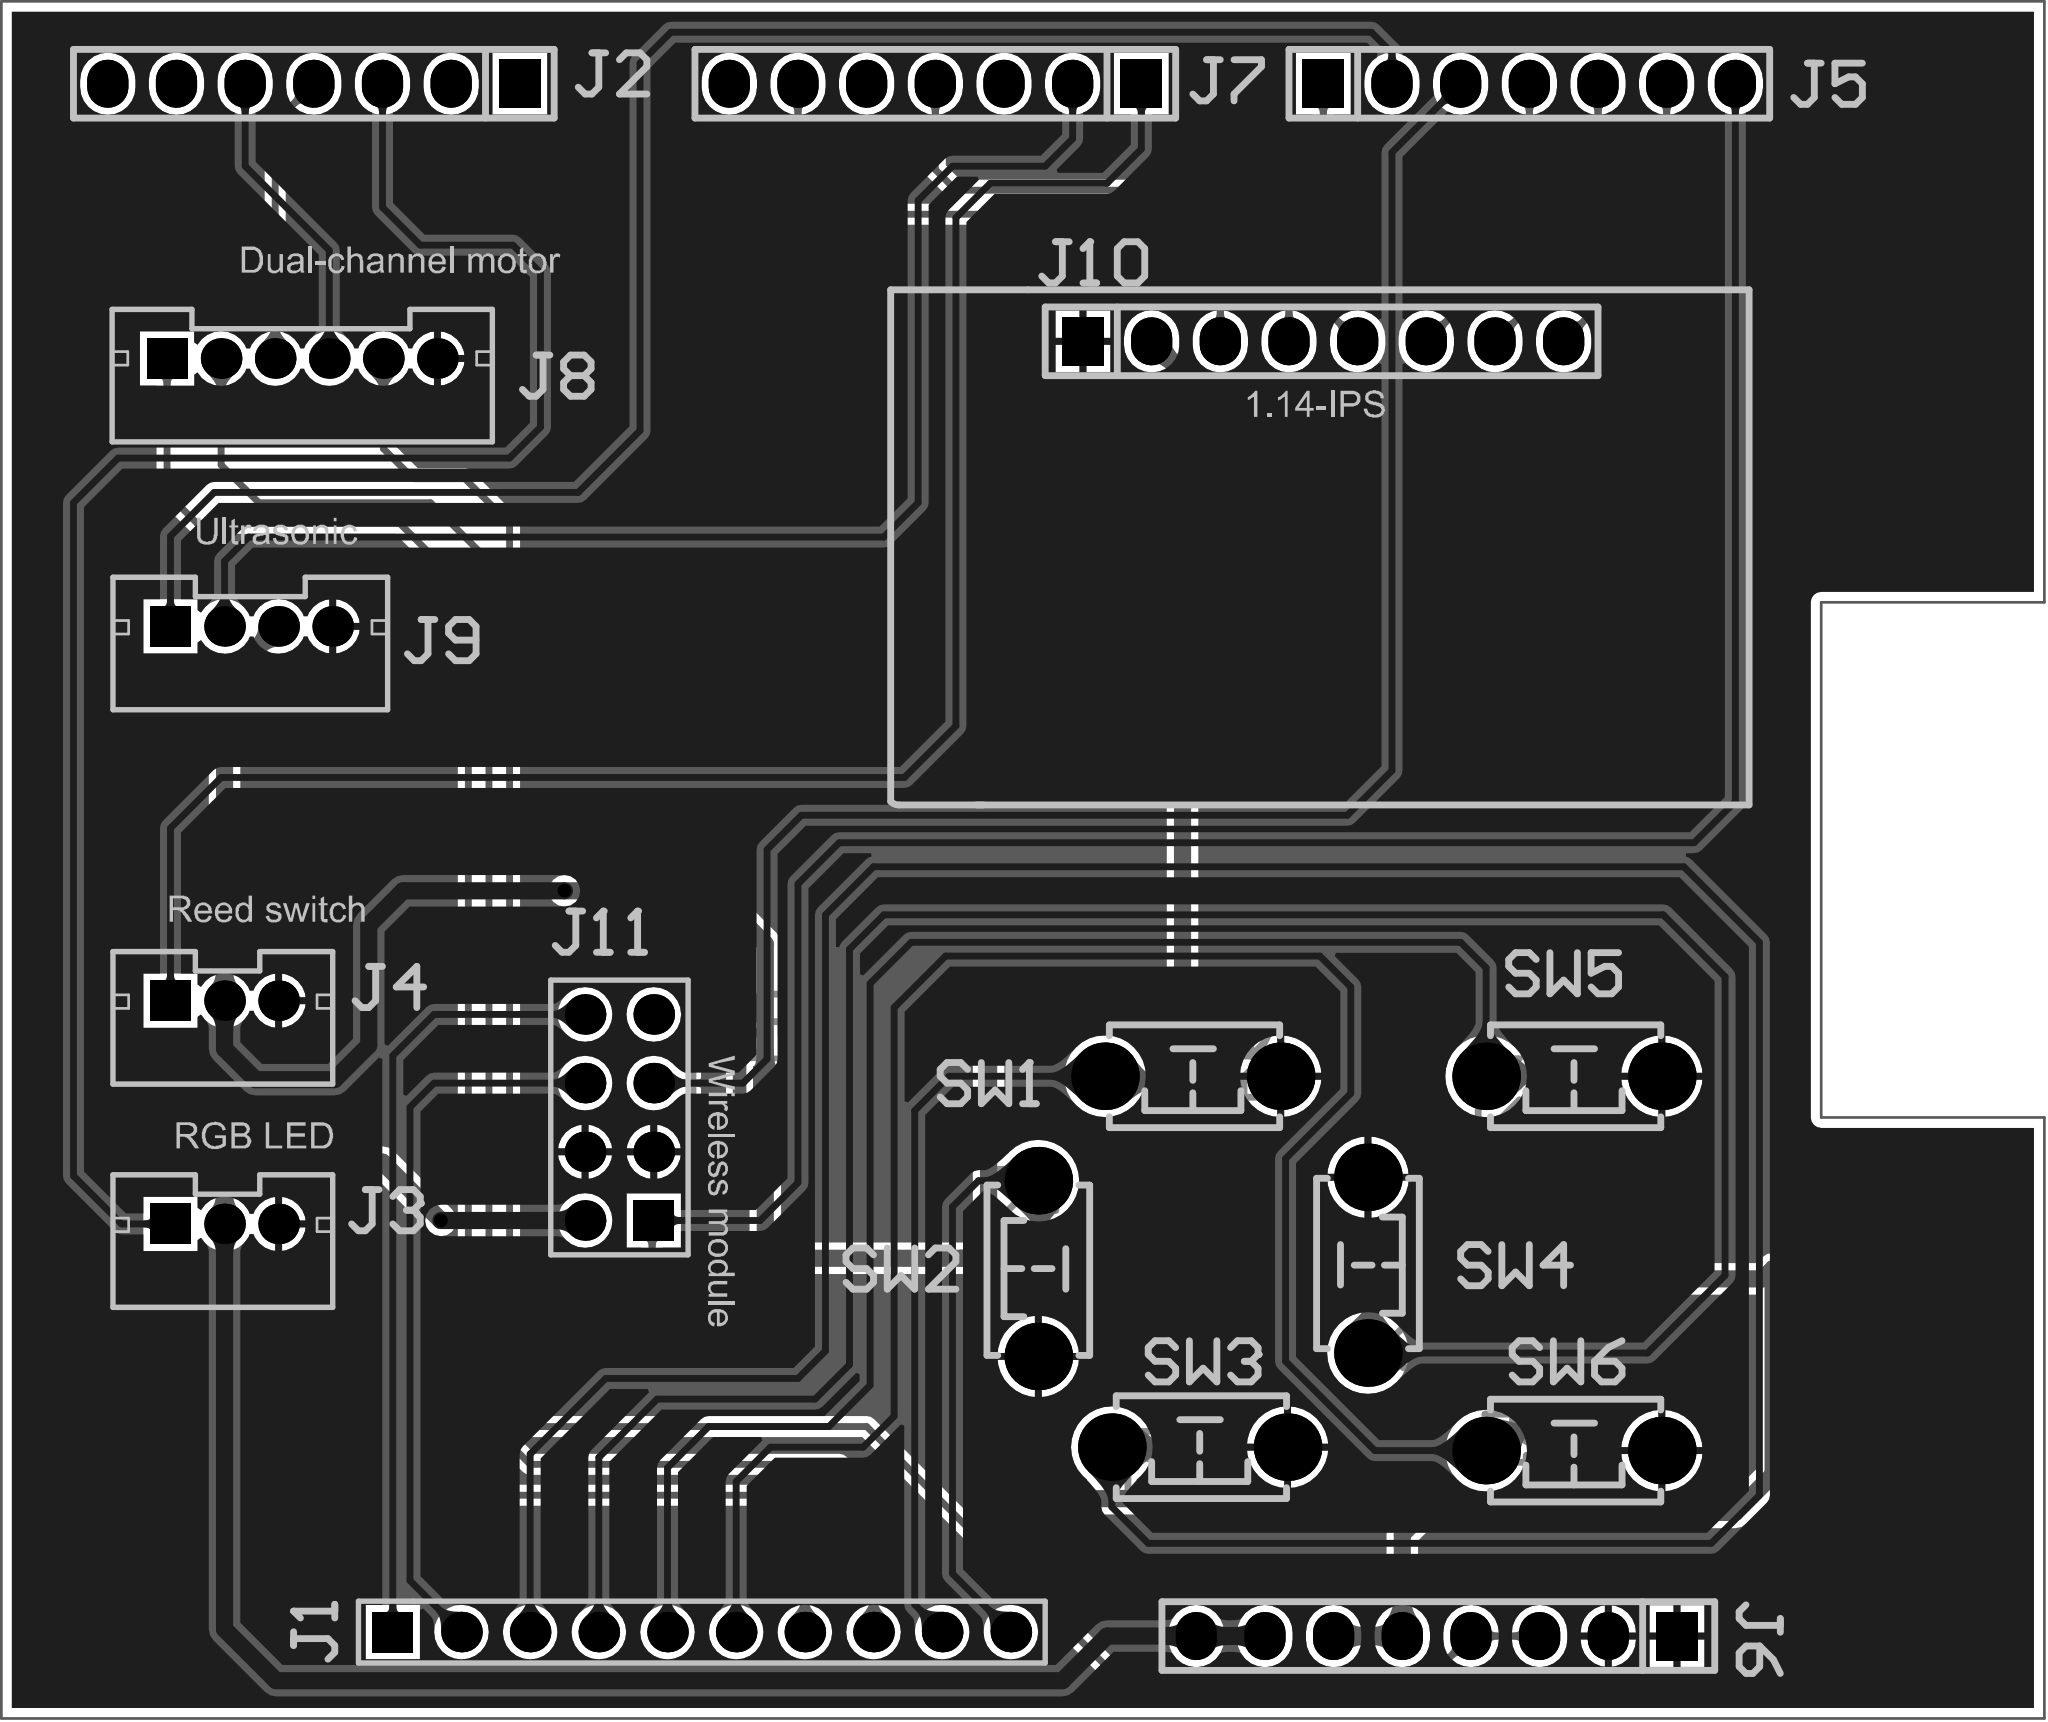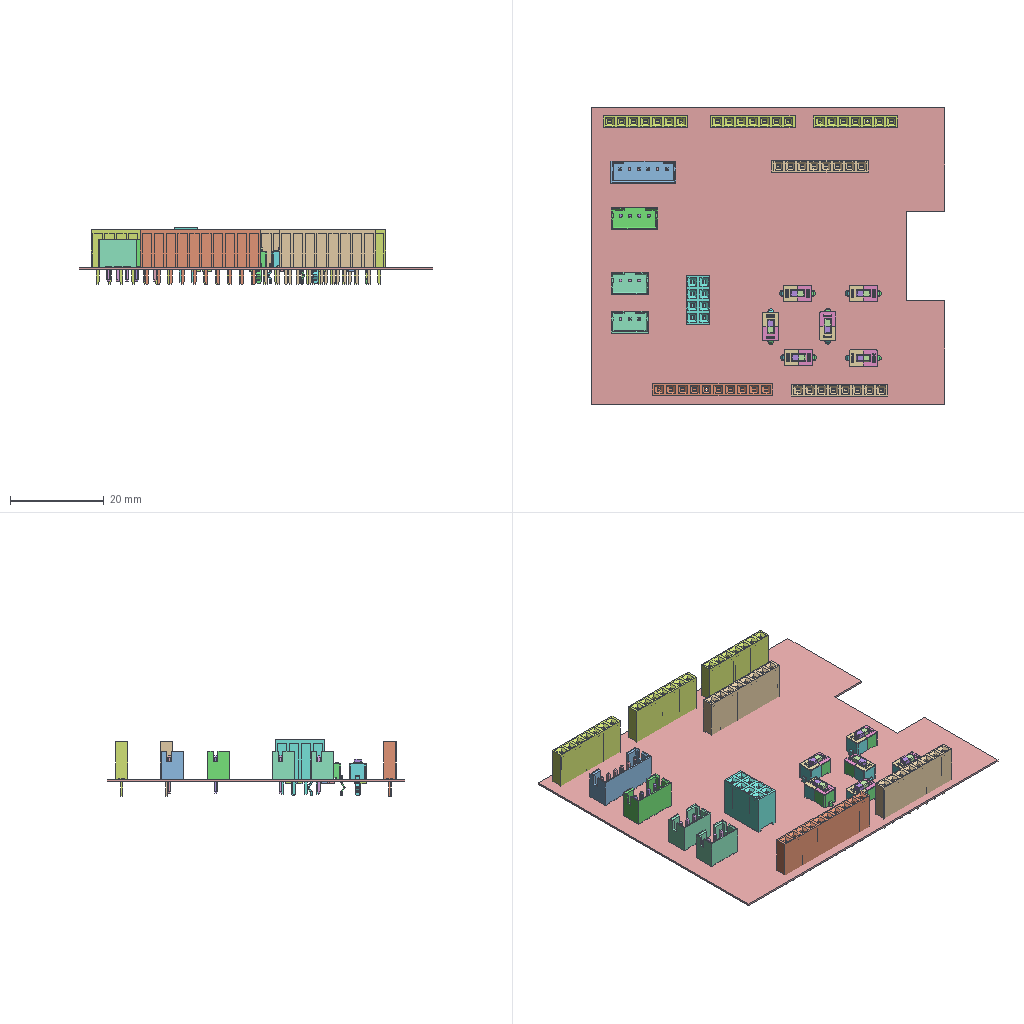Circuit board layout | Altium Designer | box 75.6 x 63.5 x 12.1 mm
Layer stack:
# Altium Designer layer stack of  (unit mm; dielectric type: 0 none, 1 core, 2 prepreg, 3 surface material)
index,name,kind,layer,copper_thickness_mm,dielectric_type,dielectric_thickness_mm,dielectric_material,dielectric_constant
0,Top Paste,other,,,,,,
1,Top Overlay,other,,,,,,
2,Top Solder,dielectric,,,3,0.0102,Solder Resist,3.5
3,Top Layer,copper,Top Layer,0.0356,,,,
4,Dielectric 1,dielectric,,,0,0.32,FR-4,4.8
5,Bottom Layer,copper,Bottom Layer,0.0356,,,,
6,Bottom Solder,dielectric,,,3,0.0102,Solder Resist,3.5
7,Bottom Overlay,other,,,,,,
8,Bottom Paste,other,,,,,,
# drill layer pairs: low layer,high layer
drill_pair,Top Layer,Bottom Layer
Part placement:
Designator,Comment,Layer,Footprint,Center-X(mm),Center-Y(mm),Rotation
SW6,3x6x5,TopLayer,TSW_DIP-3*6*4.3,97.536,46.101,180
SW5,3x6x5,TopLayer,TSW_DIP-3*6*4.3,97.536,59.944,180
SW4,3x6x5,TopLayer,TSW_DIP-3*6*4.3,89.916,52.959,270
SW3,3x6x5,TopLayer,TSW_DIP-3*6*4.3,83.693,46.228,180
SW2,3x6x5,TopLayer,TSW_DIP-3*6*4.3,77.724,52.832,90
SW1,3x6x5,TopLayer,TSW_DIP-3*6*4.3,83.439,59.944,180
R8,10K,BottomLayer,R_0805_L,66.675,59.69,180
R7,10K,BottomLayer,R_0805_L,64.389,51.689,360
R6,4.7K,BottomLayer,R_0805_L,83.058,60.706,90
R5,4.7K,BottomLayer,R_0805_L,76.835,53.213,180
R4,4.7K,BottomLayer,R_0805_L,83.566,45.273,270
R3,4.7K,BottomLayer,R_0805_L,90.998,52.451,360
R2,4.7K,BottomLayer,R_0805_L,97.282,59.055,270
R1,4.7K,BottomLayer,R_0805_L,97.536,45.913,270
J11,Female HDR2X4,TopLayer,Fe-HDR2X4/2.54-S,62.23,58.42,90
J10,CON8,TopLayer,Fe-HDR1X8/2.54-S,88.265,87.122,90
J9,PH2.0-4P,TopLayer,PH2.0-4P,48.625,76.581,360
J8,PH2.0-6P,TopLayer,PH2.0-6P,50.498,86.487,360
J7,Female HDR1X7,TopLayer,Fe-HDR1X7/2.54-S,73.914,96.647,270
J6,Female HDR1X8,TopLayer,Fe-HDR1X8/2.54-S,92.456,39.243,270
J5,Female HDR1X7,TopLayer,Fe-HDR1X7/2.54-S,95.885,96.647,90
J4,PH2.0-3P,TopLayer,PH2.0-3P,47.625,62.738,360
J3,PH2.0-3P,TopLayer,PH2.0-3P,47.625,54.483,360
J2,Female HDR1X7,TopLayer,Fe-HDR1X7/2.54-S,50.927,96.647,270
J1,Female HDR1X10,TopLayer,Fe-HDR1X10/2.54-S,65.278,39.39,90
Pad and via stacks:
# Altium Designer via and pad stacks of  (unit mm). Each distinct definition once, with the count of objects using it.
# via: kind,start_layer,end_layer,hole_mm,diameter_mm,mode(0 simple;1 top-mid-bottom;2 full stack),diameter_per_layer,count,example_net
# pad: kind,layer,hole_mm,hole_type(0 round;1 square;2 slot),plating,top_size,top_shape(1 round;2 rect;3 octagon;9 rounded rect),mid_size,bottom_size,mode,footprint,size_per_layer,count,example
pad,Multi-Layer,0.8128,0,plated,1.524x1.778,1,1.524x1.778,1.524x1.778,0,Fe-HDR1X7/2.54-S,,18,J2.7
pad,Multi-Layer,0.8128,0,plated,1.524x1.778,2,1.524x1.778,1.524x1.778,0,Fe-HDR1X7/2.54-S,,3,J2.1
pad,Multi-Layer,0.9,0,plated,1.5x1.5,1,1.5x1.5,1.5x1.5,0,Fe-HDR1X10/2.54-S,,9,J1.3
pad,Multi-Layer,0.9,0,plated,1.5x1.5,2,1.5x1.5,1.5x1.5,0,Fe-HDR1X10/2.54-S,,1,J1.1
pad,Multi-Layer,0.8,0,plated,1.5x1.5,1,1.5x1.5,1.5x1.5,0,PH2.0-3P,,4,J4.2
pad,Multi-Layer,0.8,0,plated,1.5x1.5,2,1.5x1.5,1.5x1.5,0,PH2.0-3P,,2,J4.1
pad,Multi-Layer,1.2,0,plated,2.5x2.5,1,2.5x2.5,2.5x2.5,0,TSW DIP-3*6*4.3,,12,SW1.2
pad,Multi-Layer,0.8128,0,plated,1.524x1.778,1,1.524x1.778,1.524x1.778,0,Fe-HDR1X8/2.54-S,,14,J6.7
pad,Multi-Layer,0.8128,0,plated,1.524x1.778,2,1.524x1.778,1.524x1.778,0,Fe-HDR1X8/2.54-S,,2,J6.1
pad,Multi-Layer,0.8,0,plated,1.5x1.5,1,1.5x1.5,1.5x1.5,0,PH2.0-6P,,5,J8.5
pad,Multi-Layer,0.8,0,plated,1.5x1.5,2,1.5x1.5,1.5x1.5,0,PH2.0-6P,,1,J8.1
pad,Multi-Layer,0.8,0,plated,1.5x1.5,2,1.5x1.5,1.5x1.5,0,PH2.0-4P,,1,J9.1
pad,Multi-Layer,0.8,0,plated,1.5x1.5,1,1.5x1.5,1.5x1.5,0,PH2.0-4P,,3,J9.2
pad,Multi-Layer,0.9,0,plated,1.5x1.5,2,1.5x1.5,1.5x1.5,0,Fe-HDR2X4/2.54-S,,1,J11.1
pad,Multi-Layer,0.9,0,plated,1.5x1.5,1,1.5x1.5,1.5x1.5,0,Fe-HDR2X4/2.54-S,,7,J11.2
pad,Bottom Layer,0,0,plated,1.27x0.889,2,1.27x0.889,1.27x0.889,0,R 0805_L,,16,R7.1
via,Top Layer,Bottom Layer,0.254,0.508,0,,2,5V
Copper pours:
name,layer,net,type(0 solid;1 hatched;2 none)
D,Bottom Layer,GND,0
D,Top Layer,GND,0
Design rules, without the lines most boards share:
# Altium Designer design rules of  (exported by Altium Designer, unit mm)
# columns: name | kind | enabled | priority | scope1 | scope2 | descriptor | typed fields (field=value)
SilkToSilkClearance | 55 | enabled | 1 | All | All | Silk to Silk (Clearance=0mil) (All),(All) |
SilkToSolderMaskClearance | 54 | enabled | 1 | IsPad | All | Silk To Solder Mask (Clearance=0mil) (IsPad),(All) |
MinimumSolderMaskSliver | 53 | enabled | 1 | All | All | Minimum Solder Mask Sliver (Gap=0mil) (All),(All) |
HoleToHoleClearance | 52 | enabled | 1 | All | All | Hole To Hole Clearance (Gap=10mil) (All),(All) | gap=0.254
DiffPairsRouting | 51 | enabled | 1 | All | All | Differential Pairs Uncoupled Length using the Gap Constraints (Min=10mil) (Max=10mil) (Prefered=10mil)  and Width Constraints (Min=15mil) (Max=15mil) (Prefered=15mil) (All) |
SolderMaskExpansion | 13 | enabled | 1 | All | All | Solder Mask Expansion (Expansion =4mil) (All) | expansion=0.1016
PasteMaskExpansion | 14 | enabled | 1 | All | All | Paste Mask Expansion (Expansion =0mil) (All) | expansion=0
RoutingVias | 11 | enabled | 1 | All | All | Routing Via (MinHoleWidth=28mil) (MaxHoleWidth=28mil) (PreferredHoleWidth=28mil) (MinWidth=50mil) (MaxWidth=50mil) (PreferedWidth=50mil) (All) | via_min_hole=0.7112 via_max_hole=0.7112 via_preferred_diameter=1.27 via_preferred_hole=0.7112
Width | 2 | enabled | 1 | All | All | Width Constraint (Min=10mil) (Max=30mil) (Preferred=10mil) (All) |
PolygonConnect | 20 | enabled | 1 | All | All | Polygon Connect Rule(Relief Connect )(Conductor Width=10mil) (Relief Angle=90 Angle) (Entries=4) (Air Gap Width=10mil) (All),(All) | connect_style(0=relief,1=direct,2=none)=0 relief_conductor_width=0.254 relief_entries=4
PlaneConnect | 6 | enabled | 1 | All | All | Power Plane Connect Rule(Relief Connect )(Expansion=20mil) (Conductor Width=10mil) (Air Gap=10mil) (Entries=4) (All) | relief_conductor_width=0.254 relief_entries=4 relief_expansion=0.508
Clearance | 0 | enabled | 1 | All | All | Clearance Constraint (Gap=10mil) (All),(All) | gap=0.254
Classes set for this board:
# Altium Designer classes of  (member kind: 0 net, 1 component, 2 from-to, 3 pad, 4 layer, 5 differential pair, 6 design channel, 7 polygon, 8 structure, 9 xSignal)
# columns: class name | member kind | superclass | members
Sheet1 | 1 | no | J1; J2; J3; J4; J5; J6; J7; J8; J9; J10; J11; R1; R2; R3; R4; R5; R6; R7; R8; SW1; SW2; SW3; SW4; SW5; SW6;